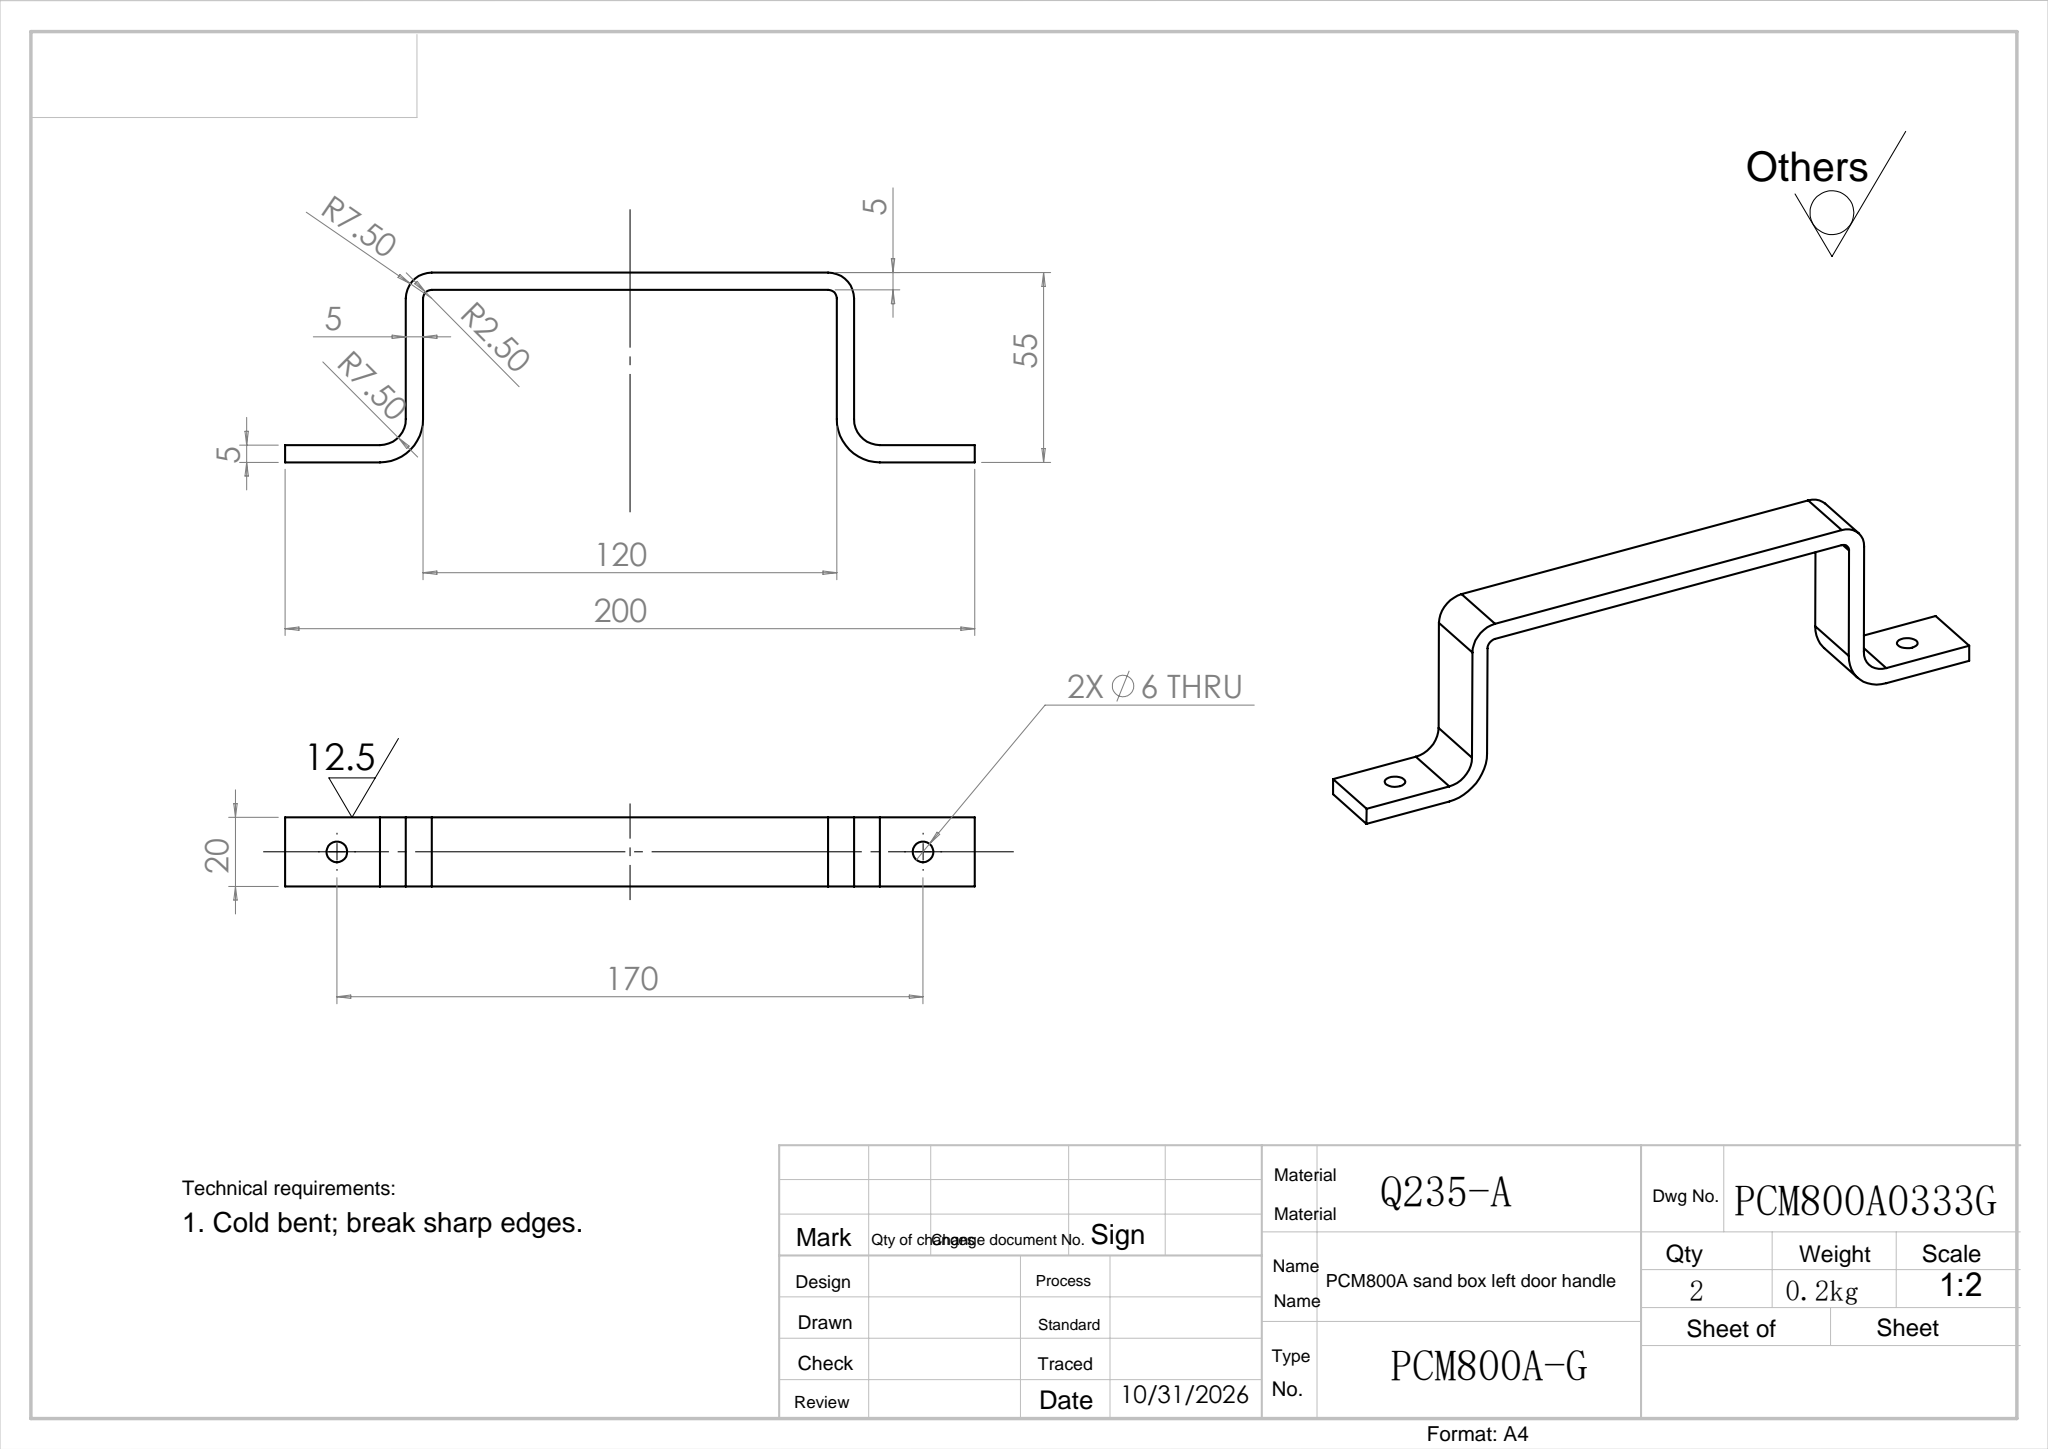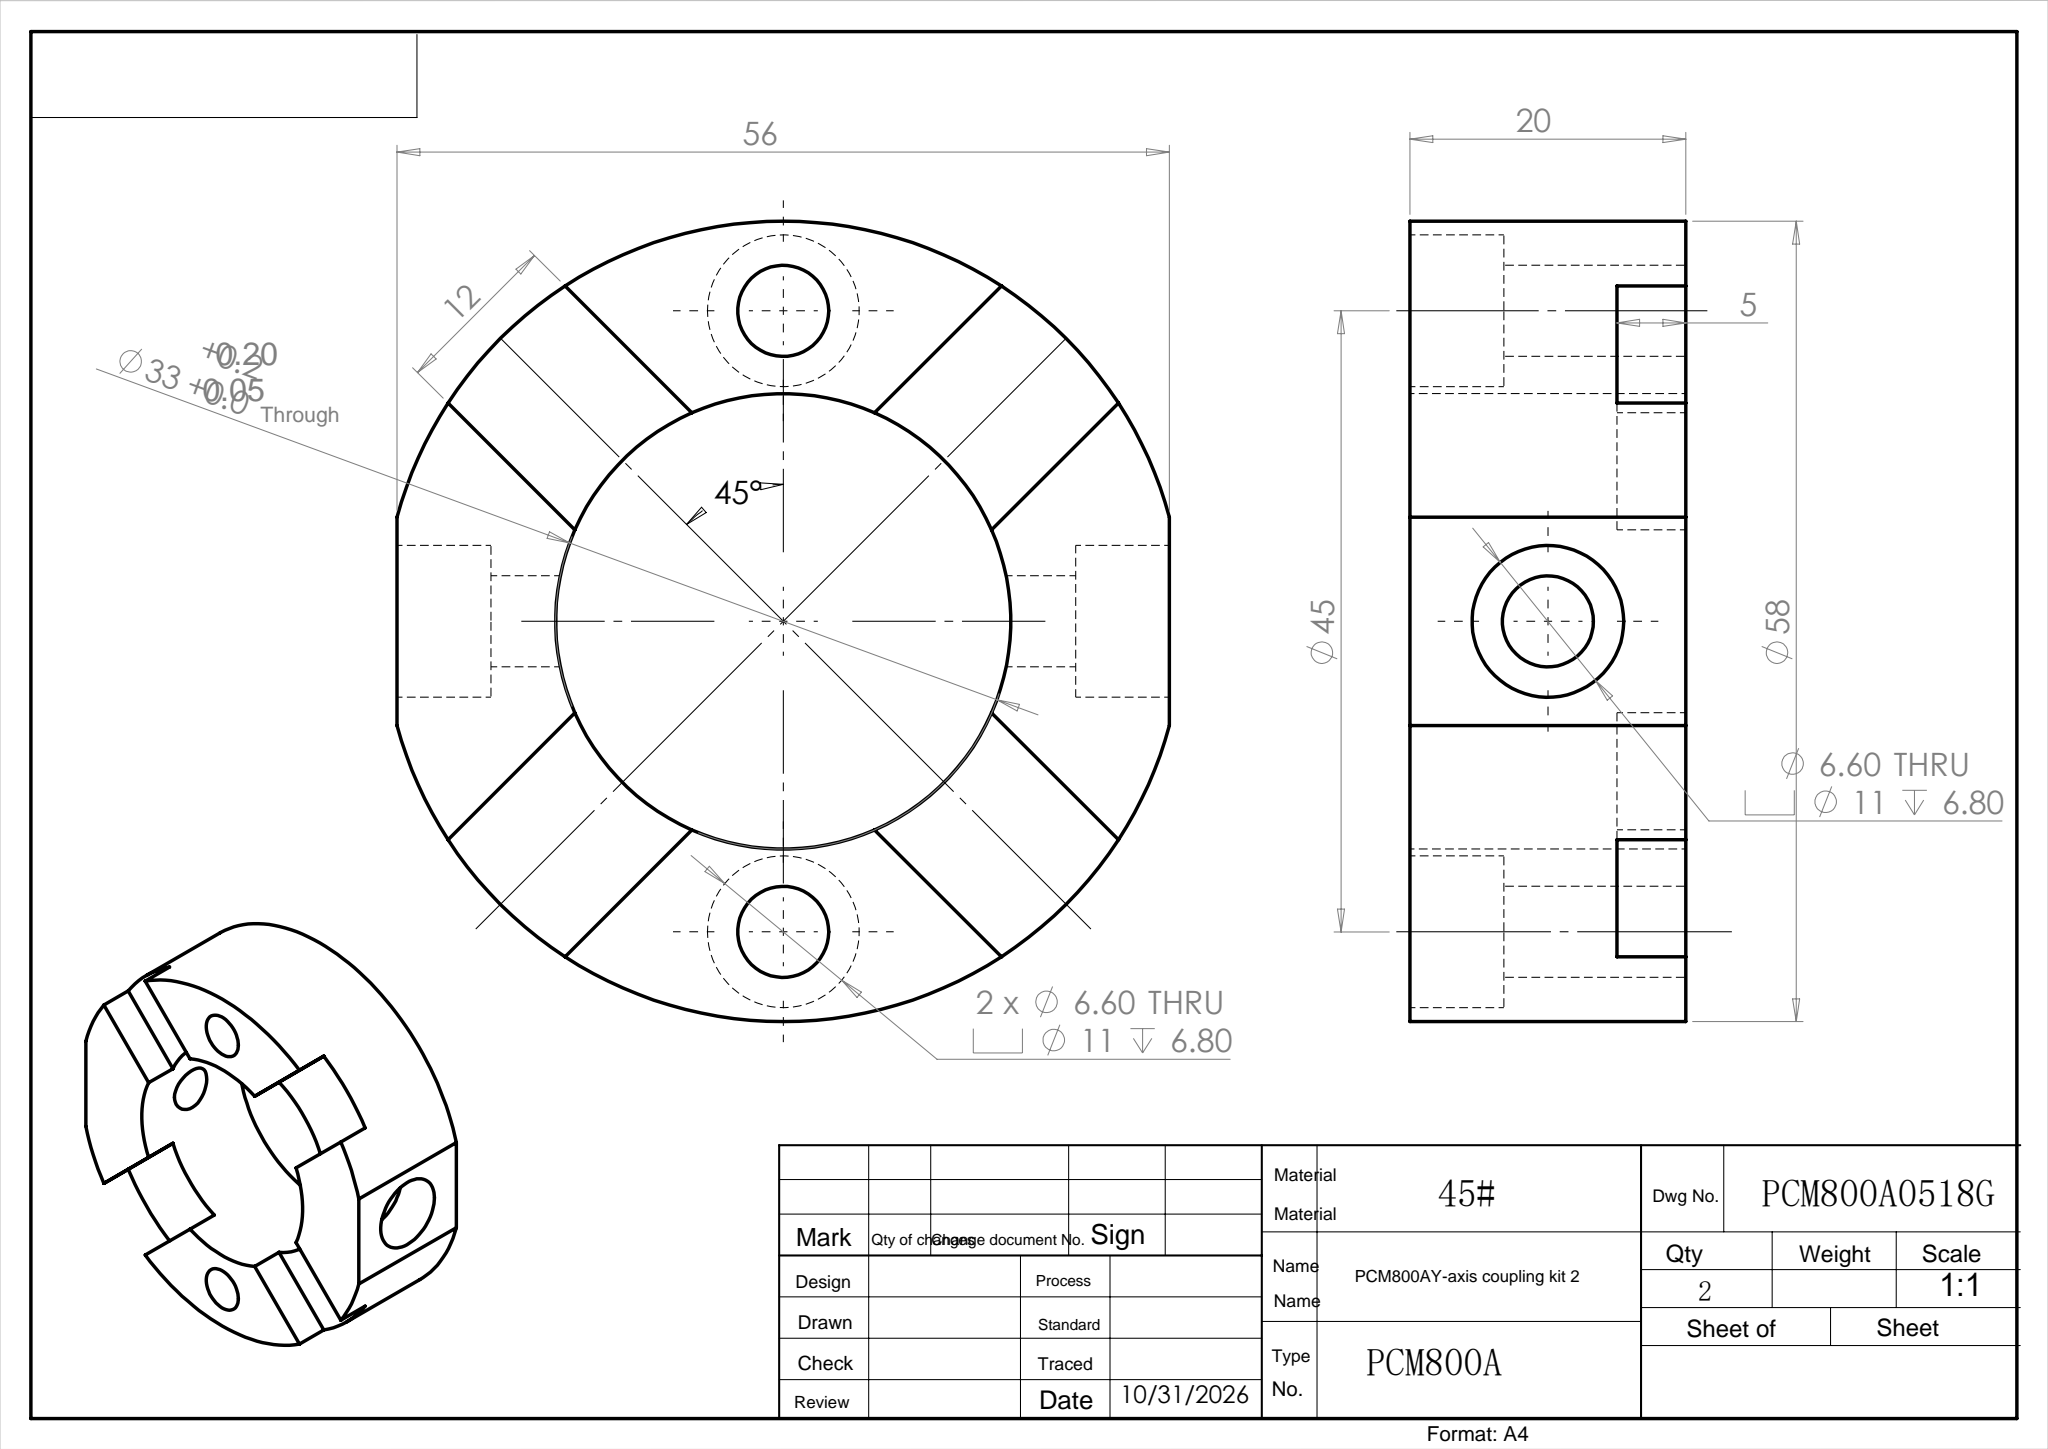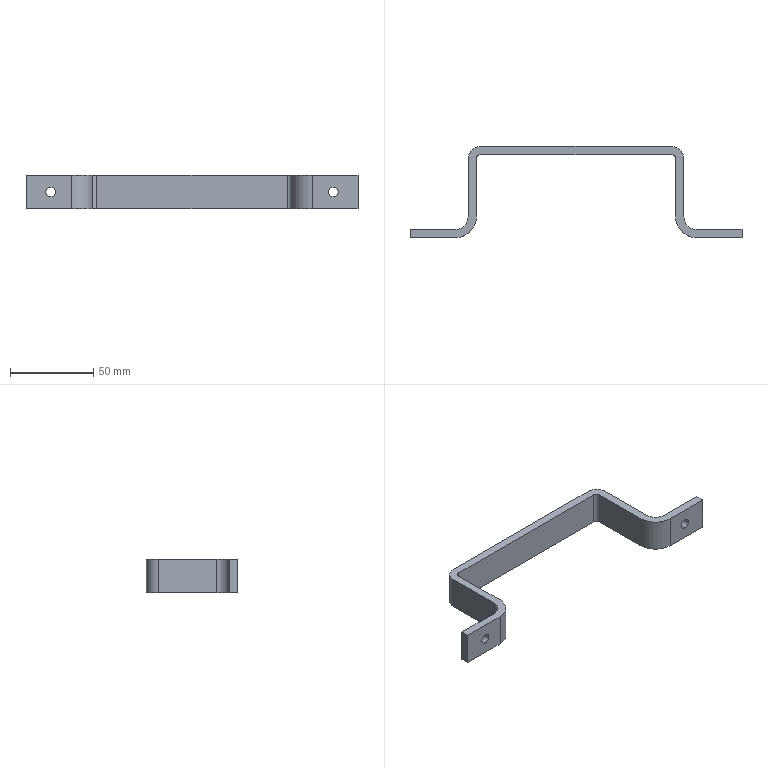Part | SolidWorks | features ExtruThin 1, ICE 1 | 1 solid | 26 faces | box 200 x 55 x 20 mm | volume 28430 mm3 | plane 14 | cylinder 12 | commonest cylinder face diameters 6 x4 15 x4 5 x2 25 x2
STEP:
#1=CARTESIAN_POINT('',(185.,0.,7.));
#2=VERTEX_POINT('',#1);
#3=CARTESIAN_POINT('',(185.,0.,13.));
#4=VERTEX_POINT('',#3);
#5=CARTESIAN_POINT('',(185.,0.,10.));
#6=DIRECTION('',(0.,1.,0.));
#7=DIRECTION('',(0.,0.,1.));
#8=AXIS2_PLACEMENT_3D('',#5,#6,#7);
#9=CIRCLE('',#8,3.);
#10=EDGE_CURVE('',#2,#4,#9,.T.);
#11=ORIENTED_EDGE('',*,*,#10,.T.);
#12=CARTESIAN_POINT('',(185.,-5.,13.));
#13=VERTEX_POINT('',#12);
#14=CARTESIAN_POINT('',(185.,50.,13.));
#15=DIRECTION('',(0.,-1.,0.));
#16=VECTOR('',#15,1000.);
#17=LINE('',#14,#16);
#18=EDGE_CURVE('',#4,#13,#17,.T.);
#19=ORIENTED_EDGE('',*,*,#18,.T.);
#20=CARTESIAN_POINT('',(185.,-5.,7.));
#21=VERTEX_POINT('',#20);
#22=CARTESIAN_POINT('',(185.,-5.,10.));
#23=DIRECTION('',(0.,-1.,0.));
#24=DIRECTION('',(0.,0.,-1.));
#25=AXIS2_PLACEMENT_3D('',#22,#23,#24);
#26=CIRCLE('',#25,3.);
#27=EDGE_CURVE('',#13,#21,#26,.T.);
#28=ORIENTED_EDGE('',*,*,#27,.T.);
#29=CARTESIAN_POINT('',(185.,50.,7.));
#30=DIRECTION('',(0.,-1.,0.));
#31=VECTOR('',#30,1000.);
#32=LINE('',#29,#31);
#33=EDGE_CURVE('',#2,#21,#32,.T.);
#34=ORIENTED_EDGE('',*,*,#33,.F.);
#35=EDGE_LOOP('',(#11,#19,#28,#34));
#36=FACE_OUTER_BOUND('',#35,.T.);
#37=CARTESIAN_POINT('',(185.,50.,10.));
#38=DIRECTION('',(0.,-1.,0.));
#39=DIRECTION('',(0.,0.,-1.));
#40=AXIS2_PLACEMENT_3D('',#37,#38,#39);
#41=CYLINDRICAL_SURFACE('',#40,3.);
#42=ADVANCED_FACE('',(#36),#41,.F.);
#43=CARTESIAN_POINT('',(15.,0.,7.));
#44=VERTEX_POINT('',#43);
#45=CARTESIAN_POINT('',(15.,0.,13.));
#46=VERTEX_POINT('',#45);
#47=CARTESIAN_POINT('',(15.,0.,10.));
#48=DIRECTION('',(0.,1.,0.));
#49=DIRECTION('',(0.,0.,1.));
#50=AXIS2_PLACEMENT_3D('',#47,#48,#49);
#51=CIRCLE('',#50,3.);
#52=EDGE_CURVE('',#44,#46,#51,.T.);
#53=ORIENTED_EDGE('',*,*,#52,.T.);
#54=CARTESIAN_POINT('',(15.,-5.,13.));
#55=VERTEX_POINT('',#54);
#56=CARTESIAN_POINT('',(15.,50.,13.));
#57=DIRECTION('',(0.,-1.,0.));
#58=VECTOR('',#57,1000.);
#59=LINE('',#56,#58);
#60=EDGE_CURVE('',#46,#55,#59,.T.);
#61=ORIENTED_EDGE('',*,*,#60,.T.);
#62=CARTESIAN_POINT('',(15.,-5.,7.));
#63=VERTEX_POINT('',#62);
#64=CARTESIAN_POINT('',(15.,-5.,10.));
#65=DIRECTION('',(0.,-1.,0.));
#66=DIRECTION('',(0.,0.,-1.));
#67=AXIS2_PLACEMENT_3D('',#64,#65,#66);
#68=CIRCLE('',#67,3.);
#69=EDGE_CURVE('',#55,#63,#68,.T.);
#70=ORIENTED_EDGE('',*,*,#69,.T.);
#71=CARTESIAN_POINT('',(15.,50.,7.));
#72=DIRECTION('',(0.,-1.,0.));
#73=VECTOR('',#72,1000.);
#74=LINE('',#71,#73);
#75=EDGE_CURVE('',#44,#63,#74,.T.);
#76=ORIENTED_EDGE('',*,*,#75,.F.);
#77=EDGE_LOOP('',(#53,#61,#70,#76));
#78=FACE_OUTER_BOUND('',#77,.T.);
#79=CARTESIAN_POINT('',(15.,50.,10.));
#80=DIRECTION('',(0.,-1.,0.));
#81=DIRECTION('',(0.,0.,-1.));
#82=AXIS2_PLACEMENT_3D('',#79,#80,#81);
#83=CYLINDRICAL_SURFACE('',#82,3.);
#84=ADVANCED_FACE('',(#78),#83,.F.);
#85=CARTESIAN_POINT('',(185.,-5.,10.));
#86=DIRECTION('',(0.,-1.,0.));
#87=DIRECTION('',(0.,0.,-1.));
#88=AXIS2_PLACEMENT_3D('',#85,#86,#87);
#89=CIRCLE('',#88,3.);
#90=EDGE_CURVE('',#21,#13,#89,.T.);
#91=ORIENTED_EDGE('',*,*,#90,.F.);
#92=ORIENTED_EDGE('',*,*,#27,.F.);
#93=EDGE_LOOP('',(#91,#92));
#94=FACE_BOUND('',#93,.T.);
#95=CARTESIAN_POINT('',(172.5,-5.,0.));
#96=VERTEX_POINT('',#95);
#97=CARTESIAN_POINT('',(200.,-5.,0.));
#98=VERTEX_POINT('',#97);
#99=CARTESIAN_POINT('',(172.5,-5.,0.));
#100=DIRECTION('',(1.,0.,0.));
#101=VECTOR('',#100,1000.);
#102=LINE('',#99,#101);
#103=EDGE_CURVE('',#96,#98,#102,.T.);
#104=ORIENTED_EDGE('',*,*,#103,.T.);
#105=CARTESIAN_POINT('',(200.,-5.,20.));
#106=VERTEX_POINT('',#105);
#107=CARTESIAN_POINT('',(200.,-5.,20.));
#108=DIRECTION('',(0.,0.,-1.));
#109=VECTOR('',#108,1000.);
#110=LINE('',#107,#109);
#111=EDGE_CURVE('',#106,#98,#110,.T.);
#112=ORIENTED_EDGE('',*,*,#111,.F.);
#113=CARTESIAN_POINT('',(172.5,-5.,20.));
#114=VERTEX_POINT('',#113);
#115=CARTESIAN_POINT('',(172.5,-5.,20.));
#116=DIRECTION('',(1.,0.,0.));
#117=VECTOR('',#116,1000.);
#118=LINE('',#115,#117);
#119=EDGE_CURVE('',#114,#106,#118,.T.);
#120=ORIENTED_EDGE('',*,*,#119,.F.);
#121=CARTESIAN_POINT('',(172.5,-5.,20.));
#122=DIRECTION('',(0.,0.,-1.));
#123=VECTOR('',#122,1000.);
#124=LINE('',#121,#123);
#125=EDGE_CURVE('',#114,#96,#124,.T.);
#126=ORIENTED_EDGE('',*,*,#125,.T.);
#127=EDGE_LOOP('',(#104,#112,#120,#126));
#128=FACE_OUTER_BOUND('',#127,.T.);
#129=CARTESIAN_POINT('',(172.5,-5.,20.));
#130=DIRECTION('',(0.,1.,0.));
#131=DIRECTION('',(0.,0.,1.));
#132=AXIS2_PLACEMENT_3D('',#129,#130,#131);
#133=PLANE('',#132);
#134=ADVANCED_FACE('',(#94,#128),#133,.F.);
#135=CARTESIAN_POINT('',(200.,0.,0.));
#136=VERTEX_POINT('',#135);
#137=CARTESIAN_POINT('',(200.,0.,0.));
#138=DIRECTION('',(0.,-1.,0.));
#139=VECTOR('',#138,1000.);
#140=LINE('',#137,#139);
#141=EDGE_CURVE('',#136,#98,#140,.T.);
#142=ORIENTED_EDGE('',*,*,#141,.F.);
#143=CARTESIAN_POINT('',(200.,0.,20.));
#144=VERTEX_POINT('',#143);
#145=CARTESIAN_POINT('',(200.,0.,20.));
#146=DIRECTION('',(0.,0.,-1.));
#147=VECTOR('',#146,1000.);
#148=LINE('',#145,#147);
#149=EDGE_CURVE('',#144,#136,#148,.T.);
#150=ORIENTED_EDGE('',*,*,#149,.F.);
#151=CARTESIAN_POINT('',(200.,0.,20.));
#152=DIRECTION('',(0.,-1.,0.));
#153=VECTOR('',#152,1000.);
#154=LINE('',#151,#153);
#155=EDGE_CURVE('',#144,#106,#154,.T.);
#156=ORIENTED_EDGE('',*,*,#155,.T.);
#157=ORIENTED_EDGE('',*,*,#111,.T.);
#158=EDGE_LOOP('',(#142,#150,#156,#157));
#159=FACE_OUTER_BOUND('',#158,.T.);
#160=CARTESIAN_POINT('',(200.,0.,20.));
#161=DIRECTION('',(1.,0.,0.));
#162=DIRECTION('',(0.,0.,-1.));
#163=AXIS2_PLACEMENT_3D('',#160,#161,#162);
#164=PLANE('',#163);
#165=ADVANCED_FACE('',(#159),#164,.T.);
#166=ORIENTED_EDGE('',*,*,#10,.F.);
#167=CARTESIAN_POINT('',(185.,0.,10.));
#168=DIRECTION('',(0.,1.,0.));
#169=DIRECTION('',(0.,0.,1.));
#170=AXIS2_PLACEMENT_3D('',#167,#168,#169);
#171=CIRCLE('',#170,3.);
#172=EDGE_CURVE('',#4,#2,#171,.T.);
#173=ORIENTED_EDGE('',*,*,#172,.F.);
#174=EDGE_LOOP('',(#166,#173));
#175=FACE_BOUND('',#174,.T.);
#176=CARTESIAN_POINT('',(172.5,0.,0.));
#177=VERTEX_POINT('',#176);
#178=CARTESIAN_POINT('',(172.5,0.,0.));
#179=DIRECTION('',(1.,0.,0.));
#180=VECTOR('',#179,1000.);
#181=LINE('',#178,#180);
#182=EDGE_CURVE('',#177,#136,#181,.T.);
#183=ORIENTED_EDGE('',*,*,#182,.F.);
#184=CARTESIAN_POINT('',(172.5,0.,20.));
#185=VERTEX_POINT('',#184);
#186=CARTESIAN_POINT('',(172.5,0.,20.));
#187=DIRECTION('',(0.,0.,-1.));
#188=VECTOR('',#187,1000.);
#189=LINE('',#186,#188);
#190=EDGE_CURVE('',#185,#177,#189,.T.);
#191=ORIENTED_EDGE('',*,*,#190,.F.);
#192=CARTESIAN_POINT('',(172.5,0.,20.));
#193=DIRECTION('',(1.,0.,0.));
#194=VECTOR('',#193,1000.);
#195=LINE('',#192,#194);
#196=EDGE_CURVE('',#185,#144,#195,.T.);
#197=ORIENTED_EDGE('',*,*,#196,.T.);
#198=ORIENTED_EDGE('',*,*,#149,.T.);
#199=EDGE_LOOP('',(#183,#191,#197,#198));
#200=FACE_OUTER_BOUND('',#199,.T.);
#201=CARTESIAN_POINT('',(172.5,0.,20.));
#202=DIRECTION('',(0.,1.,0.));
#203=DIRECTION('',(0.,0.,1.));
#204=AXIS2_PLACEMENT_3D('',#201,#202,#203);
#205=PLANE('',#204);
#206=ADVANCED_FACE('',(#175,#200),#205,.T.);
#207=CARTESIAN_POINT('',(165.,7.5,0.));
#208=VERTEX_POINT('',#207);
#209=CARTESIAN_POINT('',(172.5,7.5,0.));
#210=DIRECTION('',(0.,0.,1.));
#211=DIRECTION('',(1.,0.,0.));
#212=AXIS2_PLACEMENT_3D('',#209,#210,#211);
#213=CIRCLE('',#212,7.5);
#214=EDGE_CURVE('',#208,#177,#213,.T.);
#215=ORIENTED_EDGE('',*,*,#214,.F.);
#216=CARTESIAN_POINT('',(165.,7.5,20.));
#217=VERTEX_POINT('',#216);
#218=CARTESIAN_POINT('',(165.,7.5,20.));
#219=DIRECTION('',(0.,0.,-1.));
#220=VECTOR('',#219,1000.);
#221=LINE('',#218,#220);
#222=EDGE_CURVE('',#217,#208,#221,.T.);
#223=ORIENTED_EDGE('',*,*,#222,.F.);
#224=CARTESIAN_POINT('',(172.5,7.5,20.));
#225=DIRECTION('',(0.,0.,1.));
#226=DIRECTION('',(1.,0.,0.));
#227=AXIS2_PLACEMENT_3D('',#224,#225,#226);
#228=CIRCLE('',#227,7.5);
#229=EDGE_CURVE('',#217,#185,#228,.T.);
#230=ORIENTED_EDGE('',*,*,#229,.T.);
#231=ORIENTED_EDGE('',*,*,#190,.T.);
#232=EDGE_LOOP('',(#215,#223,#230,#231));
#233=FACE_OUTER_BOUND('',#232,.T.);
#234=CARTESIAN_POINT('',(172.5,7.5,20.));
#235=DIRECTION('',(0.,0.,-1.));
#236=DIRECTION('',(-1.,0.,0.));
#237=AXIS2_PLACEMENT_3D('',#234,#235,#236);
#238=CYLINDRICAL_SURFACE('',#237,7.5);
#239=ADVANCED_FACE('',(#233),#238,.F.);
#240=CARTESIAN_POINT('',(165.,42.5,0.));
#241=VERTEX_POINT('',#240);
#242=CARTESIAN_POINT('',(165.,42.5,0.));
#243=DIRECTION('',(0.,-1.,0.));
#244=VECTOR('',#243,1000.);
#245=LINE('',#242,#244);
#246=EDGE_CURVE('',#241,#208,#245,.T.);
#247=ORIENTED_EDGE('',*,*,#246,.F.);
#248=CARTESIAN_POINT('',(165.,42.5,20.));
#249=VERTEX_POINT('',#248);
#250=CARTESIAN_POINT('',(165.,42.5,20.));
#251=DIRECTION('',(0.,0.,-1.));
#252=VECTOR('',#251,1000.);
#253=LINE('',#250,#252);
#254=EDGE_CURVE('',#249,#241,#253,.T.);
#255=ORIENTED_EDGE('',*,*,#254,.F.);
#256=CARTESIAN_POINT('',(165.,42.5,20.));
#257=DIRECTION('',(0.,-1.,0.));
#258=VECTOR('',#257,1000.);
#259=LINE('',#256,#258);
#260=EDGE_CURVE('',#249,#217,#259,.T.);
#261=ORIENTED_EDGE('',*,*,#260,.T.);
#262=ORIENTED_EDGE('',*,*,#222,.T.);
#263=EDGE_LOOP('',(#247,#255,#261,#262));
#264=FACE_OUTER_BOUND('',#263,.T.);
#265=CARTESIAN_POINT('',(165.,42.5,20.));
#266=DIRECTION('',(1.,0.,0.));
#267=DIRECTION('',(0.,0.,-1.));
#268=AXIS2_PLACEMENT_3D('',#265,#266,#267);
#269=PLANE('',#268);
#270=ADVANCED_FACE('',(#264),#269,.T.);
#271=CARTESIAN_POINT('',(157.5,50.,0.));
#272=VERTEX_POINT('',#271);
#273=CARTESIAN_POINT('',(157.5,42.5,0.));
#274=DIRECTION('',(0.,0.,-1.));
#275=DIRECTION('',(-1.,0.,0.));
#276=AXIS2_PLACEMENT_3D('',#273,#274,#275);
#277=CIRCLE('',#276,7.5);
#278=EDGE_CURVE('',#272,#241,#277,.T.);
#279=ORIENTED_EDGE('',*,*,#278,.F.);
#280=CARTESIAN_POINT('',(157.5,50.,20.));
#281=VERTEX_POINT('',#280);
#282=CARTESIAN_POINT('',(157.5,50.,20.));
#283=DIRECTION('',(0.,0.,-1.));
#284=VECTOR('',#283,1000.);
#285=LINE('',#282,#284);
#286=EDGE_CURVE('',#281,#272,#285,.T.);
#287=ORIENTED_EDGE('',*,*,#286,.F.);
#288=CARTESIAN_POINT('',(157.5,42.5,20.));
#289=DIRECTION('',(0.,0.,-1.));
#290=DIRECTION('',(-1.,0.,0.));
#291=AXIS2_PLACEMENT_3D('',#288,#289,#290);
#292=CIRCLE('',#291,7.5);
#293=EDGE_CURVE('',#281,#249,#292,.T.);
#294=ORIENTED_EDGE('',*,*,#293,.T.);
#295=ORIENTED_EDGE('',*,*,#254,.T.);
#296=EDGE_LOOP('',(#279,#287,#294,#295));
#297=FACE_OUTER_BOUND('',#296,.T.);
#298=CARTESIAN_POINT('',(157.5,42.5,20.));
#299=DIRECTION('',(0.,0.,-1.));
#300=DIRECTION('',(-1.,0.,0.));
#301=AXIS2_PLACEMENT_3D('',#298,#299,#300);
#302=CYLINDRICAL_SURFACE('',#301,7.5);
#303=ADVANCED_FACE('',(#297),#302,.T.);
#304=CARTESIAN_POINT('',(42.5,50.,0.));
#305=VERTEX_POINT('',#304);
#306=CARTESIAN_POINT('',(42.5,50.,0.));
#307=DIRECTION('',(1.,0.,0.));
#308=VECTOR('',#307,1000.);
#309=LINE('',#306,#308);
#310=EDGE_CURVE('',#305,#272,#309,.T.);
#311=ORIENTED_EDGE('',*,*,#310,.F.);
#312=CARTESIAN_POINT('',(42.5,50.,20.));
#313=VERTEX_POINT('',#312);
#314=CARTESIAN_POINT('',(42.5,50.,20.));
#315=DIRECTION('',(0.,0.,-1.));
#316=VECTOR('',#315,1000.);
#317=LINE('',#314,#316);
#318=EDGE_CURVE('',#313,#305,#317,.T.);
#319=ORIENTED_EDGE('',*,*,#318,.F.);
#320=CARTESIAN_POINT('',(42.5,50.,20.));
#321=DIRECTION('',(1.,0.,0.));
#322=VECTOR('',#321,1000.);
#323=LINE('',#320,#322);
#324=EDGE_CURVE('',#313,#281,#323,.T.);
#325=ORIENTED_EDGE('',*,*,#324,.T.);
#326=ORIENTED_EDGE('',*,*,#286,.T.);
#327=EDGE_LOOP('',(#311,#319,#325,#326));
#328=FACE_OUTER_BOUND('',#327,.T.);
#329=CARTESIAN_POINT('',(42.5,50.,20.));
#330=DIRECTION('',(0.,1.,0.));
#331=DIRECTION('',(-1.,0.,0.));
#332=AXIS2_PLACEMENT_3D('',#329,#330,#331);
#333=PLANE('',#332);
#334=ADVANCED_FACE('',(#328),#333,.T.);
#335=CARTESIAN_POINT('',(35.,42.5,0.));
#336=VERTEX_POINT('',#335);
#337=CARTESIAN_POINT('',(42.5,42.5,0.));
#338=DIRECTION('',(0.,0.,-1.));
#339=DIRECTION('',(1.,0.,0.));
#340=AXIS2_PLACEMENT_3D('',#337,#338,#339);
#341=CIRCLE('',#340,7.5);
#342=EDGE_CURVE('',#336,#305,#341,.T.);
#343=ORIENTED_EDGE('',*,*,#342,.F.);
#344=CARTESIAN_POINT('',(35.,42.5,20.));
#345=VERTEX_POINT('',#344);
#346=CARTESIAN_POINT('',(35.,42.5,20.));
#347=DIRECTION('',(0.,0.,-1.));
#348=VECTOR('',#347,1000.);
#349=LINE('',#346,#348);
#350=EDGE_CURVE('',#345,#336,#349,.T.);
#351=ORIENTED_EDGE('',*,*,#350,.F.);
#352=CARTESIAN_POINT('',(42.5,42.5,20.));
#353=DIRECTION('',(0.,0.,-1.));
#354=DIRECTION('',(1.,0.,0.));
#355=AXIS2_PLACEMENT_3D('',#352,#353,#354);
#356=CIRCLE('',#355,7.5);
#357=EDGE_CURVE('',#345,#313,#356,.T.);
#358=ORIENTED_EDGE('',*,*,#357,.T.);
#359=ORIENTED_EDGE('',*,*,#318,.T.);
#360=EDGE_LOOP('',(#343,#351,#358,#359));
#361=FACE_OUTER_BOUND('',#360,.T.);
#362=CARTESIAN_POINT('',(42.5,42.5,20.));
#363=DIRECTION('',(0.,0.,-1.));
#364=DIRECTION('',(-1.,0.,0.));
#365=AXIS2_PLACEMENT_3D('',#362,#363,#364);
#366=CYLINDRICAL_SURFACE('',#365,7.5);
#367=ADVANCED_FACE('',(#361),#366,.T.);
#368=CARTESIAN_POINT('',(35.,7.5,0.));
#369=VERTEX_POINT('',#368);
#370=CARTESIAN_POINT('',(35.,7.5,0.));
#371=DIRECTION('',(0.,1.,0.));
#372=VECTOR('',#371,1000.);
#373=LINE('',#370,#372);
#374=EDGE_CURVE('',#369,#336,#373,.T.);
#375=ORIENTED_EDGE('',*,*,#374,.F.);
#376=CARTESIAN_POINT('',(35.,7.5,20.));
#377=VERTEX_POINT('',#376);
#378=CARTESIAN_POINT('',(35.,7.5,20.));
#379=DIRECTION('',(0.,0.,-1.));
#380=VECTOR('',#379,1000.);
#381=LINE('',#378,#380);
#382=EDGE_CURVE('',#377,#369,#381,.T.);
#383=ORIENTED_EDGE('',*,*,#382,.F.);
#384=CARTESIAN_POINT('',(35.,7.5,20.));
#385=DIRECTION('',(0.,1.,0.));
#386=VECTOR('',#385,1000.);
#387=LINE('',#384,#386);
#388=EDGE_CURVE('',#377,#345,#387,.T.);
#389=ORIENTED_EDGE('',*,*,#388,.T.);
#390=ORIENTED_EDGE('',*,*,#350,.T.);
#391=EDGE_LOOP('',(#375,#383,#389,#390));
#392=FACE_OUTER_BOUND('',#391,.T.);
#393=CARTESIAN_POINT('',(35.,7.5,20.));
#394=DIRECTION('',(-1.,0.,0.));
#395=DIRECTION('',(0.,0.,1.));
#396=AXIS2_PLACEMENT_3D('',#393,#394,#395);
#397=PLANE('',#396);
#398=ADVANCED_FACE('',(#392),#397,.T.);
#399=CARTESIAN_POINT('',(27.5,0.,0.));
#400=VERTEX_POINT('',#399);
#401=CARTESIAN_POINT('',(27.5,7.5,0.));
#402=DIRECTION('',(0.,0.,1.));
#403=DIRECTION('',(1.,0.,0.));
#404=AXIS2_PLACEMENT_3D('',#401,#402,#403);
#405=CIRCLE('',#404,7.5);
#406=EDGE_CURVE('',#400,#369,#405,.T.);
#407=ORIENTED_EDGE('',*,*,#406,.F.);
#408=CARTESIAN_POINT('',(27.5,0.,20.));
#409=VERTEX_POINT('',#408);
#410=CARTESIAN_POINT('',(27.5,0.,20.));
#411=DIRECTION('',(0.,0.,-1.));
#412=VECTOR('',#411,1000.);
#413=LINE('',#410,#412);
#414=EDGE_CURVE('',#409,#400,#413,.T.);
#415=ORIENTED_EDGE('',*,*,#414,.F.);
#416=CARTESIAN_POINT('',(27.5,7.5,20.));
#417=DIRECTION('',(0.,0.,1.));
#418=DIRECTION('',(1.,0.,0.));
#419=AXIS2_PLACEMENT_3D('',#416,#417,#418);
#420=CIRCLE('',#419,7.5);
#421=EDGE_CURVE('',#409,#377,#420,.T.);
#422=ORIENTED_EDGE('',*,*,#421,.T.);
#423=ORIENTED_EDGE('',*,*,#382,.T.);
#424=EDGE_LOOP('',(#407,#415,#422,#423));
#425=FACE_OUTER_BOUND('',#424,.T.);
#426=CARTESIAN_POINT('',(27.5,7.5,20.));
#427=DIRECTION('',(0.,0.,-1.));
#428=DIRECTION('',(-1.,0.,0.));
#429=AXIS2_PLACEMENT_3D('',#426,#427,#428);
#430=CYLINDRICAL_SURFACE('',#429,7.5);
#431=ADVANCED_FACE('',(#425),#430,.F.);
#432=ORIENTED_EDGE('',*,*,#52,.F.);
#433=CARTESIAN_POINT('',(15.,0.,10.));
#434=DIRECTION('',(0.,1.,0.));
#435=DIRECTION('',(0.,0.,1.));
#436=AXIS2_PLACEMENT_3D('',#433,#434,#435);
#437=CIRCLE('',#436,3.);
#438=EDGE_CURVE('',#46,#44,#437,.T.);
#439=ORIENTED_EDGE('',*,*,#438,.F.);
#440=EDGE_LOOP('',(#432,#439));
#441=FACE_BOUND('',#440,.T.);
#442=CARTESIAN_POINT('',(0.,0.,0.));
#443=VERTEX_POINT('',#442);
#444=CARTESIAN_POINT('',(0.,0.,0.));
#445=DIRECTION('',(1.,0.,0.));
#446=VECTOR('',#445,1000.);
#447=LINE('',#444,#446);
#448=EDGE_CURVE('',#443,#400,#447,.T.);
#449=ORIENTED_EDGE('',*,*,#448,.F.);
#450=CARTESIAN_POINT('',(0.,0.,20.));
#451=VERTEX_POINT('',#450);
#452=CARTESIAN_POINT('',(0.,0.,20.));
#453=DIRECTION('',(0.,0.,-1.));
#454=VECTOR('',#453,1000.);
#455=LINE('',#452,#454);
#456=EDGE_CURVE('',#451,#443,#455,.T.);
#457=ORIENTED_EDGE('',*,*,#456,.F.);
#458=CARTESIAN_POINT('',(0.,0.,20.));
#459=DIRECTION('',(1.,0.,0.));
#460=VECTOR('',#459,1000.);
#461=LINE('',#458,#460);
#462=EDGE_CURVE('',#451,#409,#461,.T.);
#463=ORIENTED_EDGE('',*,*,#462,.T.);
#464=ORIENTED_EDGE('',*,*,#414,.T.);
#465=EDGE_LOOP('',(#449,#457,#463,#464));
#466=FACE_OUTER_BOUND('',#465,.T.);
#467=CARTESIAN_POINT('',(0.,0.,20.));
#468=DIRECTION('',(0.,1.,0.));
#469=DIRECTION('',(0.,0.,1.));
#470=AXIS2_PLACEMENT_3D('',#467,#468,#469);
#471=PLANE('',#470);
#472=ADVANCED_FACE('',(#441,#466),#471,.T.);
#473=CARTESIAN_POINT('',(0.,-5.,0.));
#474=VERTEX_POINT('',#473);
#475=CARTESIAN_POINT('',(0.,-5.,0.));
#476=DIRECTION('',(0.,1.,0.));
#477=VECTOR('',#476,1000.);
#478=LINE('',#475,#477);
#479=EDGE_CURVE('',#474,#443,#478,.T.);
#480=ORIENTED_EDGE('',*,*,#479,.F.);
#481=CARTESIAN_POINT('',(0.,-5.,20.));
#482=VERTEX_POINT('',#481);
#483=CARTESIAN_POINT('',(0.,-5.,20.));
#484=DIRECTION('',(0.,0.,-1.));
#485=VECTOR('',#484,1000.);
#486=LINE('',#483,#485);
#487=EDGE_CURVE('',#482,#474,#486,.T.);
#488=ORIENTED_EDGE('',*,*,#487,.F.);
#489=CARTESIAN_POINT('',(0.,-5.,20.));
#490=DIRECTION('',(0.,1.,0.));
#491=VECTOR('',#490,1000.);
#492=LINE('',#489,#491);
#493=EDGE_CURVE('',#482,#451,#492,.T.);
#494=ORIENTED_EDGE('',*,*,#493,.T.);
#495=ORIENTED_EDGE('',*,*,#456,.T.);
#496=EDGE_LOOP('',(#480,#488,#494,#495));
#497=FACE_OUTER_BOUND('',#496,.T.);
#498=CARTESIAN_POINT('',(0.,-5.,20.));
#499=DIRECTION('',(-1.,0.,0.));
#500=DIRECTION('',(0.,0.,1.));
#501=AXIS2_PLACEMENT_3D('',#498,#499,#500);
#502=PLANE('',#501);
#503=ADVANCED_FACE('',(#497),#502,.T.);
#504=CARTESIAN_POINT('',(15.,-5.,10.));
#505=DIRECTION('',(0.,-1.,0.));
#506=DIRECTION('',(0.,0.,-1.));
#507=AXIS2_PLACEMENT_3D('',#504,#505,#506);
#508=CIRCLE('',#507,3.);
#509=EDGE_CURVE('',#63,#55,#508,.T.);
#510=ORIENTED_EDGE('',*,*,#509,.F.);
#511=ORIENTED_EDGE('',*,*,#69,.F.);
#512=EDGE_LOOP('',(#510,#511));
#513=FACE_BOUND('',#512,.T.);
#514=CARTESIAN_POINT('',(27.5,-5.,0.));
#515=VERTEX_POINT('',#514);
#516=CARTESIAN_POINT('',(0.,-5.,0.));
#517=DIRECTION('',(1.,0.,0.));
#518=VECTOR('',#517,1000.);
#519=LINE('',#516,#518);
#520=EDGE_CURVE('',#474,#515,#519,.T.);
#521=ORIENTED_EDGE('',*,*,#520,.T.);
#522=CARTESIAN_POINT('',(27.5,-5.,20.));
#523=VERTEX_POINT('',#522);
#524=CARTESIAN_POINT('',(27.5,-5.,20.));
#525=DIRECTION('',(0.,0.,-1.));
#526=VECTOR('',#525,1000.);
#527=LINE('',#524,#526);
#528=EDGE_CURVE('',#523,#515,#527,.T.);
#529=ORIENTED_EDGE('',*,*,#528,.F.);
#530=CARTESIAN_POINT('',(0.,-5.,20.));
#531=DIRECTION('',(1.,0.,0.));
#532=VECTOR('',#531,1000.);
#533=LINE('',#530,#532);
#534=EDGE_CURVE('',#482,#523,#533,.T.);
#535=ORIENTED_EDGE('',*,*,#534,.F.);
#536=ORIENTED_EDGE('',*,*,#487,.T.);
#537=EDGE_LOOP('',(#521,#529,#535,#536));
#538=FACE_OUTER_BOUND('',#537,.T.);
#539=CARTESIAN_POINT('',(0.,-5.,20.));
#540=DIRECTION('',(0.,1.,0.));
#541=DIRECTION('',(0.,0.,1.));
#542=AXIS2_PLACEMENT_3D('',#539,#540,#541);
#543=PLANE('',#542);
#544=ADVANCED_FACE('',(#513,#538),#543,.F.);
#545=CARTESIAN_POINT('',(40.,7.5,0.));
#546=VERTEX_POINT('',#545);
#547=CARTESIAN_POINT('',(27.5,7.5,0.));
#548=DIRECTION('',(0.,0.,1.));
#549=DIRECTION('',(1.,0.,0.));
#550=AXIS2_PLACEMENT_3D('',#547,#548,#549);
#551=CIRCLE('',#550,12.5);
#552=EDGE_CURVE('',#515,#546,#551,.T.);
#553=ORIENTED_EDGE('',*,*,#552,.T.);
#554=CARTESIAN_POINT('',(40.,7.5,20.));
#555=VERTEX_POINT('',#554);
#556=CARTESIAN_POINT('',(40.,7.5,20.));
#557=DIRECTION('',(0.,0.,-1.));
#558=VECTOR('',#557,1000.);
#559=LINE('',#556,#558);
#560=EDGE_CURVE('',#555,#546,#559,.T.);
#561=ORIENTED_EDGE('',*,*,#560,.F.);
#562=CARTESIAN_POINT('',(27.5,7.5,20.));
#563=DIRECTION('',(0.,0.,1.));
#564=DIRECTION('',(1.,0.,0.));
#565=AXIS2_PLACEMENT_3D('',#562,#563,#564);
#566=CIRCLE('',#565,12.5);
#567=EDGE_CURVE('',#523,#555,#566,.T.);
#568=ORIENTED_EDGE('',*,*,#567,.F.);
#569=ORIENTED_EDGE('',*,*,#528,.T.);
#570=EDGE_LOOP('',(#553,#561,#568,#569));
#571=FACE_OUTER_BOUND('',#570,.T.);
#572=CARTESIAN_POINT('',(27.5,7.5,20.));
#573=DIRECTION('',(0.,0.,-1.));
#574=DIRECTION('',(-1.,0.,0.));
#575=AXIS2_PLACEMENT_3D('',#572,#573,#574);
#576=CYLINDRICAL_SURFACE('',#575,12.5);
#577=ADVANCED_FACE('',(#571),#576,.T.);
#578=CARTESIAN_POINT('',(40.,42.5,0.));
#579=VERTEX_POINT('',#578);
#580=CARTESIAN_POINT('',(40.,7.5,0.));
#581=DIRECTION('',(0.,1.,0.));
#582=VECTOR('',#581,1000.);
#583=LINE('',#580,#582);
#584=EDGE_CURVE('',#546,#579,#583,.T.);
#585=ORIENTED_EDGE('',*,*,#584,.T.);
#586=CARTESIAN_POINT('',(40.,42.5,20.));
#587=VERTEX_POINT('',#586);
#588=CARTESIAN_POINT('',(40.,42.5,20.));
#589=DIRECTION('',(0.,0.,-1.));
#590=VECTOR('',#589,1000.);
#591=LINE('',#588,#590);
#592=EDGE_CURVE('',#587,#579,#591,.T.);
#593=ORIENTED_EDGE('',*,*,#592,.F.);
#594=CARTESIAN_POINT('',(40.,7.5,20.));
#595=DIRECTION('',(0.,1.,0.));
#596=VECTOR('',#595,1000.);
#597=LINE('',#594,#596);
#598=EDGE_CURVE('',#555,#587,#597,.T.);
#599=ORIENTED_EDGE('',*,*,#598,.F.);
#600=ORIENTED_EDGE('',*,*,#560,.T.);
#601=EDGE_LOOP('',(#585,#593,#599,#600));
#602=FACE_OUTER_BOUND('',#601,.T.);
#603=CARTESIAN_POINT('',(40.,7.5,20.));
#604=DIRECTION('',(-1.,0.,0.));
#605=DIRECTION('',(0.,0.,1.));
#606=AXIS2_PLACEMENT_3D('',#603,#604,#605);
#607=PLANE('',#606);
#608=ADVANCED_FACE('',(#602),#607,.F.);
#609=CARTESIAN_POINT('',(42.5,45.,0.));
#610=VERTEX_POINT('',#609);
#611=CARTESIAN_POINT('',(42.5,42.5,0.));
#612=DIRECTION('',(0.,0.,-1.));
#613=DIRECTION('',(1.,0.,0.));
#614=AXIS2_PLACEMENT_3D('',#611,#612,#613);
#615=CIRCLE('',#614,2.5);
#616=EDGE_CURVE('',#579,#610,#615,.T.);
#617=ORIENTED_EDGE('',*,*,#616,.T.);
#618=CARTESIAN_POINT('',(42.5,45.,20.));
#619=VERTEX_POINT('',#618);
#620=CARTESIAN_POINT('',(42.5,45.,20.));
#621=DIRECTION('',(0.,0.,-1.));
#622=VECTOR('',#621,1000.);
#623=LINE('',#620,#622);
#624=EDGE_CURVE('',#619,#610,#623,.T.);
#625=ORIENTED_EDGE('',*,*,#624,.F.);
#626=CARTESIAN_POINT('',(42.5,42.5,20.));
#627=DIRECTION('',(0.,0.,-1.));
#628=DIRECTION('',(1.,0.,0.));
#629=AXIS2_PLACEMENT_3D('',#626,#627,#628);
#630=CIRCLE('',#629,2.5);
#631=EDGE_CURVE('',#587,#619,#630,.T.);
#632=ORIENTED_EDGE('',*,*,#631,.F.);
#633=ORIENTED_EDGE('',*,*,#592,.T.);
#634=EDGE_LOOP('',(#617,#625,#632,#633));
#635=FACE_OUTER_BOUND('',#634,.T.);
#636=CARTESIAN_POINT('',(42.5,42.5,20.));
#637=DIRECTION('',(0.,0.,-1.));
#638=DIRECTION('',(-1.,0.,0.));
#639=AXIS2_PLACEMENT_3D('',#636,#637,#638);
#640=CYLINDRICAL_SURFACE('',#639,2.5);
#641=ADVANCED_FACE('',(#635),#640,.F.);
#642=CARTESIAN_POINT('',(157.5,45.,0.));
#643=VERTEX_POINT('',#642);
#644=CARTESIAN_POINT('',(42.5,45.,0.));
#645=DIRECTION('',(1.,0.,0.));
#646=VECTOR('',#645,1000.);
#647=LINE('',#644,#646);
#648=EDGE_CURVE('',#610,#643,#647,.T.);
#649=ORIENTED_EDGE('',*,*,#648,.T.);
#650=CARTESIAN_POINT('',(157.5,45.,20.));
#651=VERTEX_POINT('',#650);
#652=CARTESIAN_POINT('',(157.5,45.,20.));
#653=DIRECTION('',(0.,0.,-1.));
#654=VECTOR('',#653,1000.);
#655=LINE('',#652,#654);
#656=EDGE_CURVE('',#651,#643,#655,.T.);
#657=ORIENTED_EDGE('',*,*,#656,.F.);
#658=CARTESIAN_POINT('',(42.5,45.,20.));
#659=DIRECTION('',(1.,0.,0.));
#660=VECTOR('',#659,1000.);
#661=LINE('',#658,#660);
#662=EDGE_CURVE('',#619,#651,#661,.T.);
#663=ORIENTED_EDGE('',*,*,#662,.F.);
#664=ORIENTED_EDGE('',*,*,#624,.T.);
#665=EDGE_LOOP('',(#649,#657,#663,#664));
#666=FACE_OUTER_BOUND('',#665,.T.);
#667=CARTESIAN_POINT('',(42.5,45.,20.));
#668=DIRECTION('',(0.,1.,0.));
#669=DIRECTION('',(-1.,0.,0.));
#670=AXIS2_PLACEMENT_3D('',#667,#668,#669);
#671=PLANE('',#670);
#672=ADVANCED_FACE('',(#666),#671,.F.);
#673=CARTESIAN_POINT('',(160.,42.5,0.));
#674=VERTEX_POINT('',#673);
#675=CARTESIAN_POINT('',(157.5,42.5,0.));
#676=DIRECTION('',(0.,0.,-1.));
#677=DIRECTION('',(1.,0.,0.));
#678=AXIS2_PLACEMENT_3D('',#675,#676,#677);
#679=CIRCLE('',#678,2.5);
#680=EDGE_CURVE('',#643,#674,#679,.T.);
#681=ORIENTED_EDGE('',*,*,#680,.T.);
#682=CARTESIAN_POINT('',(160.,42.5,20.));
#683=VERTEX_POINT('',#682);
#684=CARTESIAN_POINT('',(160.,42.5,20.));
#685=DIRECTION('',(0.,0.,-1.));
#686=VECTOR('',#685,1000.);
#687=LINE('',#684,#686);
#688=EDGE_CURVE('',#683,#674,#687,.T.);
#689=ORIENTED_EDGE('',*,*,#688,.F.);
#690=CARTESIAN_POINT('',(157.5,42.5,20.));
#691=DIRECTION('',(0.,0.,-1.));
#692=DIRECTION('',(1.,0.,0.));
#693=AXIS2_PLACEMENT_3D('',#690,#691,#692);
#694=CIRCLE('',#693,2.5);
#695=EDGE_CURVE('',#651,#683,#694,.T.);
#696=ORIENTED_EDGE('',*,*,#695,.F.);
#697=ORIENTED_EDGE('',*,*,#656,.T.);
#698=EDGE_LOOP('',(#681,#689,#696,#697));
#699=FACE_OUTER_BOUND('',#698,.T.);
#700=CARTESIAN_POINT('',(157.5,42.5,20.));
#701=DIRECTION('',(0.,0.,-1.));
#702=DIRECTION('',(-1.,0.,0.));
#703=AXIS2_PLACEMENT_3D('',#700,#701,#702);
#704=CYLINDRICAL_SURFACE('',#703,2.5);
#705=ADVANCED_FACE('',(#699),#704,.F.);
#706=CARTESIAN_POINT('',(160.,7.5,0.));
#707=VERTEX_POINT('',#706);
#708=CARTESIAN_POINT('',(160.,42.5,0.));
#709=DIRECTION('',(0.,-1.,0.));
#710=VECTOR('',#709,1000.);
#711=LINE('',#708,#710);
#712=EDGE_CURVE('',#674,#707,#711,.T.);
#713=ORIENTED_EDGE('',*,*,#712,.T.);
#714=CARTESIAN_POINT('',(160.,7.5,20.));
#715=VERTEX_POINT('',#714);
#716=CARTESIAN_POINT('',(160.,7.5,20.));
#717=DIRECTION('',(0.,0.,-1.));
#718=VECTOR('',#717,1000.);
#719=LINE('',#716,#718);
#720=EDGE_CURVE('',#715,#707,#719,.T.);
#721=ORIENTED_EDGE('',*,*,#720,.F.);
#722=CARTESIAN_POINT('',(160.,42.5,20.));
#723=DIRECTION('',(0.,-1.,0.));
#724=VECTOR('',#723,1000.);
#725=LINE('',#722,#724);
#726=EDGE_CURVE('',#683,#715,#725,.T.);
#727=ORIENTED_EDGE('',*,*,#726,.F.);
#728=ORIENTED_EDGE('',*,*,#688,.T.);
#729=EDGE_LOOP('',(#713,#721,#727,#728));
#730=FACE_OUTER_BOUND('',#729,.T.);
#731=CARTESIAN_POINT('',(160.,42.5,20.));
#732=DIRECTION('',(1.,0.,0.));
#733=DIRECTION('',(0.,0.,-1.));
#734=AXIS2_PLACEMENT_3D('',#731,#732,#733);
#735=PLANE('',#734);
#736=ADVANCED_FACE('',(#730),#735,.F.);
#737=CARTESIAN_POINT('',(172.5,7.5,0.));
#738=DIRECTION('',(0.,0.,1.));
#739=DIRECTION('',(1.,0.,0.));
#740=AXIS2_PLACEMENT_3D('',#737,#738,#739);
#741=CIRCLE('',#740,12.5);
#742=EDGE_CURVE('',#707,#96,#741,.T.);
#743=ORIENTED_EDGE('',*,*,#742,.T.);
#744=ORIENTED_EDGE('',*,*,#125,.F.);
#745=CARTESIAN_POINT('',(172.5,7.5,20.));
#746=DIRECTION('',(0.,0.,1.));
#747=DIRECTION('',(1.,0.,0.));
#748=AXIS2_PLACEMENT_3D('',#745,#746,#747);
#749=CIRCLE('',#748,12.5);
#750=EDGE_CURVE('',#715,#114,#749,.T.);
#751=ORIENTED_EDGE('',*,*,#750,.F.);
#752=ORIENTED_EDGE('',*,*,#720,.T.);
#753=EDGE_LOOP('',(#743,#744,#751,#752));
#754=FACE_OUTER_BOUND('',#753,.T.);
#755=CARTESIAN_POINT('',(172.5,7.5,20.));
#756=DIRECTION('',(0.,0.,-1.));
#757=DIRECTION('',(-1.,0.,0.));
#758=AXIS2_PLACEMENT_3D('',#755,#756,#757);
#759=CYLINDRICAL_SURFACE('',#758,12.5);
#760=ADVANCED_FACE('',(#754),#759,.T.);
#761=ORIENTED_EDGE('',*,*,#119,.T.);
#762=ORIENTED_EDGE('',*,*,#155,.F.);
#763=ORIENTED_EDGE('',*,*,#196,.F.);
#764=ORIENTED_EDGE('',*,*,#229,.F.);
#765=ORIENTED_EDGE('',*,*,#260,.F.);
#766=ORIENTED_EDGE('',*,*,#293,.F.);
#767=ORIENTED_EDGE('',*,*,#324,.F.);
#768=ORIENTED_EDGE('',*,*,#357,.F.);
#769=ORIENTED_EDGE('',*,*,#388,.F.);
#770=ORIENTED_EDGE('',*,*,#421,.F.);
#771=ORIENTED_EDGE('',*,*,#462,.F.);
#772=ORIENTED_EDGE('',*,*,#493,.F.);
#773=ORIENTED_EDGE('',*,*,#534,.T.);
#774=ORIENTED_EDGE('',*,*,#567,.T.);
#775=ORIENTED_EDGE('',*,*,#598,.T.);
#776=ORIENTED_EDGE('',*,*,#631,.T.);
#777=ORIENTED_EDGE('',*,*,#662,.T.);
#778=ORIENTED_EDGE('',*,*,#695,.T.);
#779=ORIENTED_EDGE('',*,*,#726,.T.);
#780=ORIENTED_EDGE('',*,*,#750,.T.);
#781=EDGE_LOOP('',(#761,#762,#763,#764,#765,#766,#767,#768,#769,#770,#771,#772,#773,#774,#775,#776,#777,#778,#779,#780));
#782=FACE_OUTER_BOUND('',#781,.T.);
#783=CARTESIAN_POINT('',(172.5,7.5,20.));
#784=DIRECTION('',(0.,0.,1.));
#785=DIRECTION('',(1.,0.,0.));
#786=AXIS2_PLACEMENT_3D('',#783,#784,#785);
#787=PLANE('',#786);
#788=ADVANCED_FACE('',(#782),#787,.T.);
#789=ORIENTED_EDGE('',*,*,#103,.F.);
#790=ORIENTED_EDGE('',*,*,#742,.F.);
#791=ORIENTED_EDGE('',*,*,#712,.F.);
#792=ORIENTED_EDGE('',*,*,#680,.F.);
#793=ORIENTED_EDGE('',*,*,#648,.F.);
#794=ORIENTED_EDGE('',*,*,#616,.F.);
#795=ORIENTED_EDGE('',*,*,#584,.F.);
#796=ORIENTED_EDGE('',*,*,#552,.F.);
#797=ORIENTED_EDGE('',*,*,#520,.F.);
#798=ORIENTED_EDGE('',*,*,#479,.T.);
#799=ORIENTED_EDGE('',*,*,#448,.T.);
#800=ORIENTED_EDGE('',*,*,#406,.T.);
#801=ORIENTED_EDGE('',*,*,#374,.T.);
#802=ORIENTED_EDGE('',*,*,#342,.T.);
#803=ORIENTED_EDGE('',*,*,#310,.T.);
#804=ORIENTED_EDGE('',*,*,#278,.T.);
#805=ORIENTED_EDGE('',*,*,#246,.T.);
#806=ORIENTED_EDGE('',*,*,#214,.T.);
#807=ORIENTED_EDGE('',*,*,#182,.T.);
#808=ORIENTED_EDGE('',*,*,#141,.T.);
#809=EDGE_LOOP('',(#789,#790,#791,#792,#793,#794,#795,#796,#797,#798,#799,#800,#801,#802,#803,#804,#805,#806,#807,#808));
#810=FACE_OUTER_BOUND('',#809,.T.);
#811=CARTESIAN_POINT('',(172.5,7.5,0.));
#812=DIRECTION('',(0.,0.,1.));
#813=DIRECTION('',(1.,0.,0.));
#814=AXIS2_PLACEMENT_3D('',#811,#812,#813);
#815=PLANE('',#814);
#816=ADVANCED_FACE('',(#810),#815,.F.);
#817=ORIENTED_EDGE('',*,*,#60,.F.);
#818=ORIENTED_EDGE('',*,*,#438,.T.);
#819=ORIENTED_EDGE('',*,*,#75,.T.);
#820=ORIENTED_EDGE('',*,*,#509,.T.);
#821=EDGE_LOOP('',(#817,#818,#819,#820));
#822=FACE_OUTER_BOUND('',#821,.T.);
#823=CARTESIAN_POINT('',(15.,50.,10.));
#824=DIRECTION('',(0.,-1.,0.));
#825=DIRECTION('',(0.,0.,-1.));
#826=AXIS2_PLACEMENT_3D('',#823,#824,#825);
#827=CYLINDRICAL_SURFACE('',#826,3.);
#828=ADVANCED_FACE('',(#822),#827,.F.);
#829=ORIENTED_EDGE('',*,*,#18,.F.);
#830=ORIENTED_EDGE('',*,*,#172,.T.);
#831=ORIENTED_EDGE('',*,*,#33,.T.);
#832=ORIENTED_EDGE('',*,*,#90,.T.);
#833=EDGE_LOOP('',(#829,#830,#831,#832));
#834=FACE_OUTER_BOUND('',#833,.T.);
#835=CARTESIAN_POINT('',(185.,50.,10.));
#836=DIRECTION('',(0.,-1.,0.));
#837=DIRECTION('',(0.,0.,-1.));
#838=AXIS2_PLACEMENT_3D('',#835,#836,#837);
#839=CYLINDRICAL_SURFACE('',#838,3.);
#840=ADVANCED_FACE('',(#834),#839,.F.);
#841=CLOSED_SHELL('',(#42,#84,#134,#165,#206,#239,#270,#303,#334,#367,#398,#431,#472,#503,#544,#577,#608,#641,#672,#705,#736,#760,#788,#816,#828,#840));
#842=MANIFOLD_SOLID_BREP('',#841);
#843=CARTESIAN_POINT('',(0.,0.,0.));
#844=DIRECTION('',(0.,0.,1.));
#845=DIRECTION('',(1.,0.,0.));
#846=AXIS2_PLACEMENT_3D('',#843,#844,#845);
#847=(LENGTH_UNIT()NAMED_UNIT(*)SI_UNIT(.MILLI.,.METRE.));
#848=UNCERTAINTY_MEASURE_WITH_UNIT(LENGTH_MEASURE(0.00001),#847,'','');
#849=(NAMED_UNIT(*)PLANE_ANGLE_UNIT()SI_UNIT($,.RADIAN.));
#850=(NAMED_UNIT(*)SI_UNIT($,.STERADIAN.)SOLID_ANGLE_UNIT());
#851=(GEOMETRIC_REPRESENTATION_CONTEXT(3)GLOBAL_UNCERTAINTY_ASSIGNED_CONTEXT((#848))GLOBAL_UNIT_ASSIGNED_CONTEXT((#847,#849,#850))REPRESENTATION_CONTEXT('',''));
#852=ADVANCED_BREP_SHAPE_REPRESENTATION('',(#842,#846),#851);